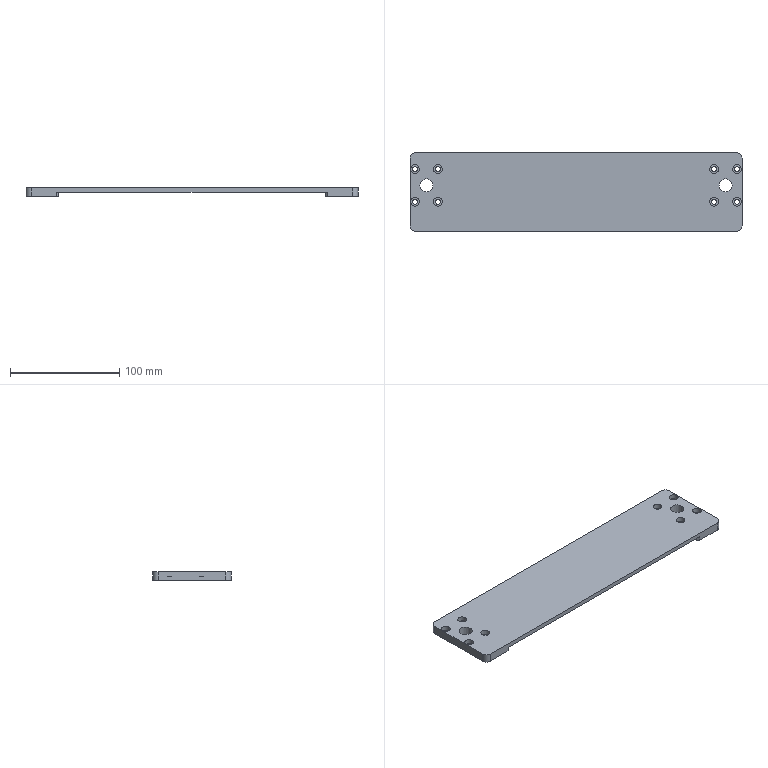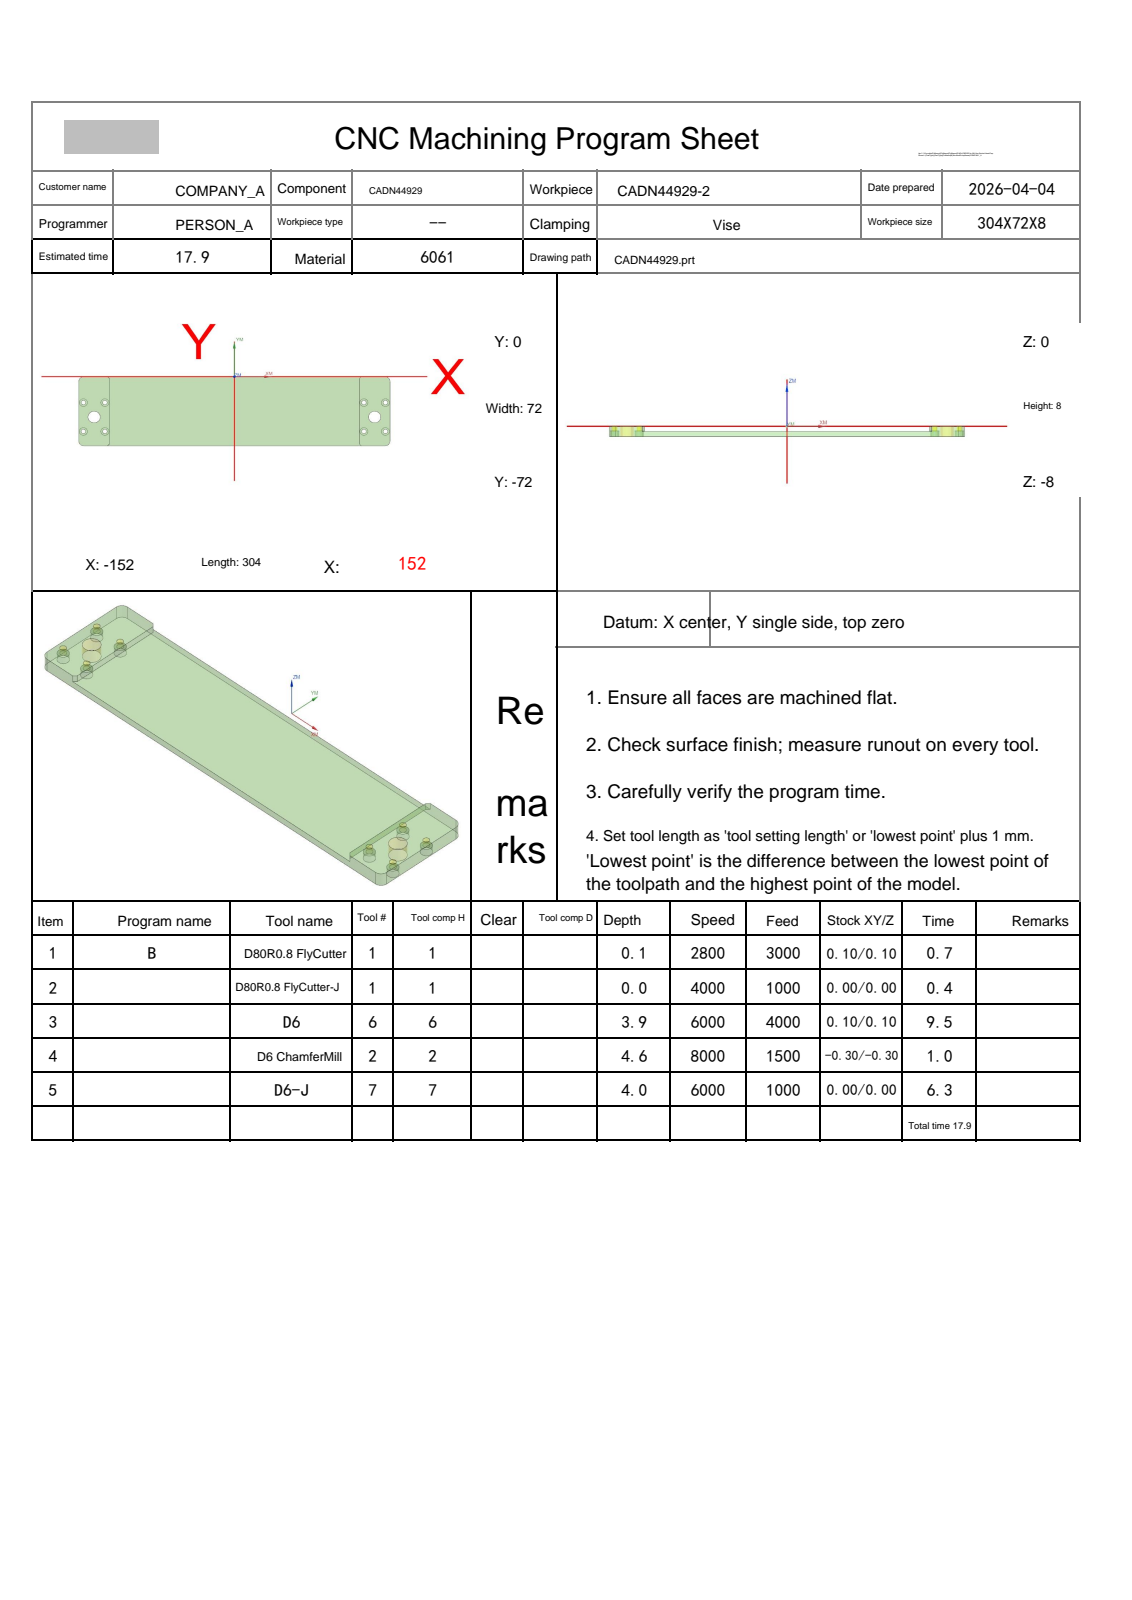NC program | NX | posted by the shop | part box 304 x 72 x 8 mm
Whole program, first 1815 of 1961 lines:
%
O0001
(Machine time: 18.92 MIN)
(===Total Tool:4===)
(T1=D80R0.8 FlyCutter D=80.  R=0.8  D-  H01 Z=0.    )
(T6=D6      D=6.   R=0.   D-  H06 Z=-3.9  )
(T2=D6 ChamferMill   D=6.   R=0.   D-  H02 Z=-4.6  )
(T7=D6-J    D=6.   R=0.   D7  H07 Z=-4.   )
G80 G90 G17 G49 G40
G91 G28 Z0
M01
N1 T01 M06
(D80R0.8 FlyCutter  D=80. R=0.8 H=01 ce=0.10 di=0.10)
G00 G90 G54 X204.097 Y-36. M03 S2800
G43 H01 Z20.
M08
Z3.525
G01 Z1.525 F3000.
X192.097
X-192.097
X-204.097
Z3.525
G00 X204.097
Z3.05
G01 Z1.05
X192.097
X-192.097
X-204.097
Z3.05
G00 X204.097
Z2.575
G01 Z.575
X192.097
X-192.097
X-204.097
Z2.575
G00 X204.097
Z2.1
G01 Z.1
X192.097
X-192.097
X-204.097
Z2.1
G00 Z20.
G91 G28 Z0.0
M05
M09
G91 G28 Z0.0
M01
N2 T01 M06
(D80R0.8 FlyCutter-J  D=80. R=0.8 H=01 ce=0.00 di=0.00)
G00 G90 G54 X203.999 Y-36. M03 S4000
G43 H01 Z20.
M08
Z2.
G01 Z0.0 F1000.
X191.999
X-191.999
X-203.999
Z2.
G00 Z20.
G91 G28 Z0.0
M05
M09
G91 G28 Z0.0
M01
N3 T06 M06
(D6  D=6. R=0. H=06 ce=0.10 di=0.10)
G00 G90 G54 X0.0 Y-78. M03 S6000
G43 H06 Z11.8
M08
Z1.013
G01 Z-.488 F4000.
Y-74.94
X-122.556
X-118.9 Y-71.284
Y-.716
X-122.556 Y2.94
X122.556
X118.9 Y-.716
Y-71.284
X122.556 Y-74.94
X1.821
G02 X1.322 Y-74.673 I.001 J.6
G01 X-1.322 Y-70.707
G03 X-1.82 Y-70.44 I-.499 J-.333
G01 X-113.803
G02 X-114.4 Y-69.843 I.003 J.6
G01 Y-2.157
G02 X-113.803 Y-1.56 I.6 J-.003
G01 X113.803
G02 X114.4 Y-2.157 I-.003 J-.6
G01 Y-69.843
G02 X113.803 Y-70.44 I-.6 J.003
G01 X1.821
G02 X1.322 Y-70.173 I.001 J.6
G01 X-1.322 Y-66.207
G03 X-1.821 Y-65.94 I-.499 J-.333
G01 X-109.303
G02 X-109.9 Y-65.343 I.003 J.6
G01 Y-6.657
G02 X-109.303 Y-6.06 I.6 J-.003
G01 X109.303
G02 X109.9 Y-6.657 I-.003 J-.6
G01 Y-65.343
G02 X109.303 Y-65.94 I-.6 J.003
G01 X1.821
G02 X1.322 Y-65.673 I.001 J.6
G01 X-1.322 Y-61.707
G03 X-1.821 Y-61.44 I-.499 J-.333
G01 X-104.804
G02 X-105.4 Y-60.844 I.004 J.6
G01 Y-11.156
G02 X-104.804 Y-10.56 I.6 J-.004
G01 X104.804
G02 X105.4 Y-11.156 I-.004 J-.6
G01 Y-60.844
G02 X104.804 Y-61.44 I-.6 J.004
G01 X1.821
G02 X1.322 Y-61.173 I.001 J.6
G01 X-1.322 Y-57.207
G03 X-1.821 Y-56.94 I-.499 J-.333
G01 X-100.304
G02 X-100.9 Y-56.344 I.004 J.6
G01 Y-15.656
G02 X-100.304 Y-15.06 I.6 J-.004
G01 X100.304
G02 X100.9 Y-15.656 I-.004 J-.6
G01 Y-56.344
G02 X100.304 Y-56.94 I-.6 J.004
G01 X1.821
G02 X1.322 Y-56.673 I.001 J.6
G01 X-1.322 Y-52.707
G03 X-1.821 Y-52.44 I-.499 J-.333
G01 X-95.804
G02 X-96.4 Y-51.844 I.004 J.6
G01 Y-20.156
G02 X-95.804 Y-19.56 I.6 J-.004
G01 X95.804
G02 X96.4 Y-20.156 I-.004 J-.6
G01 Y-51.844
G02 X95.804 Y-52.44 I-.6 J.004
G01 X1.821
G02 X1.322 Y-52.173 I.001 J.6
G01 X-1.322 Y-48.207
G03 X-1.821 Y-47.94 I-.499 J-.333
G01 X-91.305
G02 X-91.9 Y-47.345 I.005 J.6
G01 Y-24.655
G02 X-91.305 Y-24.06 I.6 J-.004
G01 X91.305
G02 X91.9 Y-24.655 I-.005 J-.6
G01 Y-47.345
G02 X91.305 Y-47.94 I-.6 J.004
G01 X1.821
G02 X1.322 Y-47.673 I.001 J.6
G01 X-1.322 Y-43.707
G03 X-1.821 Y-43.44 I-.499 J-.333
G01 X-86.805
G02 X-87.4 Y-42.845 I.005 J.6
G01 Y-29.155
G02 X-86.805 Y-28.56 I.6 J-.005
G01 X86.805
G02 X87.4 Y-29.155 I-.005 J-.6
G01 Y-42.845
G02 X86.805 Y-43.44 I-.6 J.005
G01 X1.821
G02 X1.322 Y-43.173 I.001 J.6
G01 X-1.322 Y-39.207
G03 X-1.821 Y-38.94 I-.499 J-.333
G01 X-82.305
G02 X-82.9 Y-38.345 I.005 J.6
G01 Y-33.655
G02 X-82.305 Y-33.06 I.6 J-.005
G01 X82.305
G02 X82.9 Y-33.655 I-.005 J-.6
G01 Y-38.345
G02 X82.305 Y-38.94 I-.6 J.005
G01 X1.598
G02 X1.175 Y-38.765 I.001 J.6
G01 X-1.174 Y-36.416
G03 X-1.599 Y-36.24 I-.424 J-.424
G01 X-79.963
G02 X-80.2 Y-36. I.003 J.24
G01 Y-35.997
G02 X-79.963 Y-35.76 I.24 J-.003
G01 X79.963
G02 X80.2 Y-36. I-.003 J-.24
G01 Y-36.003
G02 X79.963 Y-36.24 I-.24 J.003
G01 X0.0
X-.5
Y-39.24
Z1.013
G00 X0.0 Y-78.
Z.525
G01 Z-.975
Y-74.94
X-122.556
X-118.9 Y-71.284
Y-.716
X-122.556 Y2.94
X122.556
X118.9 Y-.716
Y-71.284
X122.556 Y-74.94
X1.821
G02 X1.322 Y-74.673 I.001 J.6
G01 X-1.322 Y-70.707
G03 X-1.82 Y-70.44 I-.499 J-.333
G01 X-113.803
G02 X-114.4 Y-69.843 I.003 J.6
G01 Y-2.157
G02 X-113.803 Y-1.56 I.6 J-.003
G01 X113.803
G02 X114.4 Y-2.157 I-.003 J-.6
G01 Y-69.843
G02 X113.803 Y-70.44 I-.6 J.003
G01 X1.821
G02 X1.322 Y-70.173 I.001 J.6
G01 X-1.322 Y-66.207
G03 X-1.821 Y-65.94 I-.499 J-.333
G01 X-109.303
G02 X-109.9 Y-65.343 I.003 J.6
G01 Y-6.657
G02 X-109.303 Y-6.06 I.6 J-.003
G01 X109.303
G02 X109.9 Y-6.657 I-.003 J-.6
G01 Y-65.343
G02 X109.303 Y-65.94 I-.6 J.003
G01 X1.821
G02 X1.322 Y-65.673 I.001 J.6
G01 X-1.322 Y-61.707
G03 X-1.821 Y-61.44 I-.499 J-.333
G01 X-104.804
G02 X-105.4 Y-60.844 I.004 J.6
G01 Y-11.156
G02 X-104.804 Y-10.56 I.6 J-.004
G01 X104.804
G02 X105.4 Y-11.156 I-.004 J-.6
G01 Y-60.844
G02 X104.804 Y-61.44 I-.6 J.004
G01 X1.821
G02 X1.322 Y-61.173 I.001 J.6
G01 X-1.322 Y-57.207
G03 X-1.821 Y-56.94 I-.499 J-.333
G01 X-100.304
G02 X-100.9 Y-56.344 I.004 J.6
G01 Y-15.656
G02 X-100.304 Y-15.06 I.6 J-.004
G01 X100.304
G02 X100.9 Y-15.656 I-.004 J-.6
G01 Y-56.344
G02 X100.304 Y-56.94 I-.6 J.004
G01 X1.821
G02 X1.322 Y-56.673 I.001 J.6
G01 X-1.322 Y-52.707
G03 X-1.821 Y-52.44 I-.499 J-.333
G01 X-95.804
G02 X-96.4 Y-51.844 I.004 J.6
G01 Y-20.156
G02 X-95.804 Y-19.56 I.6 J-.004
G01 X95.804
G02 X96.4 Y-20.156 I-.004 J-.6
G01 Y-51.844
G02 X95.804 Y-52.44 I-.6 J.004
G01 X1.821
G02 X1.322 Y-52.173 I.001 J.6
G01 X-1.322 Y-48.207
G03 X-1.821 Y-47.94 I-.499 J-.333
G01 X-91.305
G02 X-91.9 Y-47.345 I.005 J.6
G01 Y-24.655
G02 X-91.305 Y-24.06 I.6 J-.004
G01 X91.305
G02 X91.9 Y-24.655 I-.005 J-.6
G01 Y-47.345
G02 X91.305 Y-47.94 I-.6 J.004
G01 X1.821
G02 X1.322 Y-47.673 I.001 J.6
G01 X-1.322 Y-43.707
G03 X-1.821 Y-43.44 I-.499 J-.333
G01 X-86.805
G02 X-87.4 Y-42.845 I.005 J.6
G01 Y-29.155
G02 X-86.805 Y-28.56 I.6 J-.005
G01 X86.805
G02 X87.4 Y-29.155 I-.005 J-.6
G01 Y-42.845
G02 X86.805 Y-43.44 I-.6 J.005
G01 X1.821
G02 X1.322 Y-43.173 I.001 J.6
G01 X-1.322 Y-39.207
G03 X-1.821 Y-38.94 I-.499 J-.333
G01 X-82.305
G02 X-82.9 Y-38.345 I.005 J.6
G01 Y-33.655
G02 X-82.305 Y-33.06 I.6 J-.005
G01 X82.305
G02 X82.9 Y-33.655 I-.005 J-.6
G01 Y-38.345
G02 X82.305 Y-38.94 I-.6 J.005
G01 X1.598
G02 X1.175 Y-38.765 I.001 J.6
G01 X-1.174 Y-36.416
G03 X-1.599 Y-36.24 I-.424 J-.424
G01 X-79.963
G02 X-80.2 Y-36. I.003 J.24
G01 Y-35.997
G02 X-79.963 Y-35.76 I.24 J-.003
G01 X79.963
G02 X80.2 Y-36. I-.003 J-.24
G01 Y-36.003
G02 X79.963 Y-36.24 I-.24 J.003
G01 X0.0
X-.5
Y-39.24
Z.525
G00 X0.0 Y-78.
Z.038
G01 Z-1.463
Y-74.94
X-122.556
X-118.9 Y-71.284
Y-.716
X-122.556 Y2.94
X122.556
X118.9 Y-.716
Y-71.284
X122.556 Y-74.94
X1.821
G02 X1.322 Y-74.673 I.001 J.6
G01 X-1.322 Y-70.707
G03 X-1.82 Y-70.44 I-.499 J-.333
G01 X-113.803
G02 X-114.4 Y-69.843 I.003 J.6
G01 Y-2.157
G02 X-113.803 Y-1.56 I.6 J-.003
G01 X113.803
G02 X114.4 Y-2.157 I-.003 J-.6
G01 Y-69.843
G02 X113.803 Y-70.44 I-.6 J.003
G01 X1.821
G02 X1.322 Y-70.173 I.001 J.6
G01 X-1.322 Y-66.207
G03 X-1.821 Y-65.94 I-.499 J-.333
G01 X-109.303
G02 X-109.9 Y-65.343 I.003 J.6
G01 Y-6.657
G02 X-109.303 Y-6.06 I.6 J-.003
G01 X109.303
G02 X109.9 Y-6.657 I-.003 J-.6
G01 Y-65.343
G02 X109.303 Y-65.94 I-.6 J.003
G01 X1.821
G02 X1.322 Y-65.673 I.001 J.6
G01 X-1.322 Y-61.707
G03 X-1.821 Y-61.44 I-.499 J-.333
G01 X-104.804
G02 X-105.4 Y-60.844 I.004 J.6
G01 Y-11.156
G02 X-104.804 Y-10.56 I.6 J-.004
G01 X104.804
G02 X105.4 Y-11.156 I-.004 J-.6
G01 Y-60.844
G02 X104.804 Y-61.44 I-.6 J.004
G01 X1.821
G02 X1.322 Y-61.173 I.001 J.6
G01 X-1.322 Y-57.207
G03 X-1.821 Y-56.94 I-.499 J-.333
G01 X-100.304
G02 X-100.9 Y-56.344 I.004 J.6
G01 Y-15.656
G02 X-100.304 Y-15.06 I.6 J-.004
G01 X100.304
G02 X100.9 Y-15.656 I-.004 J-.6
G01 Y-56.344
G02 X100.304 Y-56.94 I-.6 J.004
G01 X1.821
G02 X1.322 Y-56.673 I.001 J.6
G01 X-1.322 Y-52.707
G03 X-1.821 Y-52.44 I-.499 J-.333
G01 X-95.804
G02 X-96.4 Y-51.844 I.004 J.6
G01 Y-20.156
G02 X-95.804 Y-19.56 I.6 J-.004
G01 X95.804
G02 X96.4 Y-20.156 I-.004 J-.6
G01 Y-51.844
G02 X95.804 Y-52.44 I-.6 J.004
G01 X1.821
G02 X1.322 Y-52.173 I.001 J.6
G01 X-1.322 Y-48.207
G03 X-1.821 Y-47.94 I-.499 J-.333
G01 X-91.305
G02 X-91.9 Y-47.345 I.005 J.6
G01 Y-24.655
G02 X-91.305 Y-24.06 I.6 J-.004
G01 X91.305
G02 X91.9 Y-24.655 I-.005 J-.6
G01 Y-47.345
G02 X91.305 Y-47.94 I-.6 J.004
G01 X1.821
G02 X1.322 Y-47.673 I.001 J.6
G01 X-1.322 Y-43.707
G03 X-1.821 Y-43.44 I-.499 J-.333
G01 X-86.805
G02 X-87.4 Y-42.845 I.005 J.6
G01 Y-29.155
G02 X-86.805 Y-28.56 I.6 J-.005
G01 X86.805
G02 X87.4 Y-29.155 I-.005 J-.6
G01 Y-42.845
G02 X86.805 Y-43.44 I-.6 J.005
G01 X1.821
G02 X1.322 Y-43.173 I.001 J.6
G01 X-1.322 Y-39.207
G03 X-1.821 Y-38.94 I-.499 J-.333
G01 X-82.305
G02 X-82.9 Y-38.345 I.005 J.6
G01 Y-33.655
G02 X-82.305 Y-33.06 I.6 J-.005
G01 X82.305
G02 X82.9 Y-33.655 I-.005 J-.6
G01 Y-38.345
G02 X82.305 Y-38.94 I-.6 J.005
G01 X1.598
G02 X1.175 Y-38.765 I.001 J.6
G01 X-1.174 Y-36.416
G03 X-1.599 Y-36.24 I-.424 J-.424
G01 X-79.963
G02 X-80.2 Y-36. I.003 J.24
G01 Y-35.997
G02 X-79.963 Y-35.76 I.24 J-.003
G01 X79.963
G02 X80.2 Y-36. I-.003 J-.24
G01 Y-36.003
G02 X79.963 Y-36.24 I-.24 J.003
G01 X0.0
X-.5
Y-39.24
Z.038
G00 X0.0 Y-78.
Z-.45
G01 Z-1.95
Y-74.94
X-122.556
X-118.9 Y-71.284
Y-.716
X-122.556 Y2.94
X122.556
X118.9 Y-.716
Y-71.284
X122.556 Y-74.94
X1.821
G02 X1.322 Y-74.673 I.001 J.6
G01 X-1.322 Y-70.707
G03 X-1.82 Y-70.44 I-.499 J-.333
G01 X-113.803
G02 X-114.4 Y-69.843 I.003 J.6
G01 Y-2.157
G02 X-113.803 Y-1.56 I.6 J-.003
G01 X113.803
G02 X114.4 Y-2.157 I-.003 J-.6
G01 Y-69.843
G02 X113.803 Y-70.44 I-.6 J.003
G01 X1.821
G02 X1.322 Y-70.173 I.001 J.6
G01 X-1.322 Y-66.207
G03 X-1.821 Y-65.94 I-.499 J-.333
G01 X-109.303
G02 X-109.9 Y-65.343 I.003 J.6
G01 Y-6.657
G02 X-109.303 Y-6.06 I.6 J-.003
G01 X109.303
G02 X109.9 Y-6.657 I-.003 J-.6
G01 Y-65.343
G02 X109.303 Y-65.94 I-.6 J.003
G01 X1.821
G02 X1.322 Y-65.673 I.001 J.6
G01 X-1.322 Y-61.707
G03 X-1.821 Y-61.44 I-.499 J-.333
G01 X-104.804
G02 X-105.4 Y-60.844 I.004 J.6
G01 Y-11.156
G02 X-104.804 Y-10.56 I.6 J-.004
G01 X104.804
G02 X105.4 Y-11.156 I-.004 J-.6
G01 Y-60.844
G02 X104.804 Y-61.44 I-.6 J.004
G01 X1.821
G02 X1.322 Y-61.173 I.001 J.6
G01 X-1.322 Y-57.207
G03 X-1.821 Y-56.94 I-.499 J-.333
G01 X-100.304
G02 X-100.9 Y-56.344 I.004 J.6
G01 Y-15.656
G02 X-100.304 Y-15.06 I.6 J-.004
G01 X100.304
G02 X100.9 Y-15.656 I-.004 J-.6
G01 Y-56.344
G02 X100.304 Y-56.94 I-.6 J.004
G01 X1.821
G02 X1.322 Y-56.673 I.001 J.6
G01 X-1.322 Y-52.707
G03 X-1.821 Y-52.44 I-.499 J-.333
G01 X-95.804
G02 X-96.4 Y-51.844 I.004 J.6
G01 Y-20.156
G02 X-95.804 Y-19.56 I.6 J-.004
G01 X95.804
G02 X96.4 Y-20.156 I-.004 J-.6
G01 Y-51.844
G02 X95.804 Y-52.44 I-.6 J.004
G01 X1.821
G02 X1.322 Y-52.173 I.001 J.6
G01 X-1.322 Y-48.207
G03 X-1.821 Y-47.94 I-.499 J-.333
G01 X-91.305
G02 X-91.9 Y-47.345 I.005 J.6
G01 Y-24.655
G02 X-91.305 Y-24.06 I.6 J-.004
G01 X91.305
G02 X91.9 Y-24.655 I-.005 J-.6
G01 Y-47.345
G02 X91.305 Y-47.94 I-.6 J.004
G01 X1.821
G02 X1.322 Y-47.673 I.001 J.6
G01 X-1.322 Y-43.707
G03 X-1.821 Y-43.44 I-.499 J-.333
G01 X-86.805
G02 X-87.4 Y-42.845 I.005 J.6
G01 Y-29.155
G02 X-86.805 Y-28.56 I.6 J-.005
G01 X86.805
G02 X87.4 Y-29.155 I-.005 J-.6
G01 Y-42.845
G02 X86.805 Y-43.44 I-.6 J.005
G01 X1.821
G02 X1.322 Y-43.173 I.001 J.6
G01 X-1.322 Y-39.207
G03 X-1.821 Y-38.94 I-.499 J-.333
G01 X-82.305
G02 X-82.9 Y-38.345 I.005 J.6
G01 Y-33.655
G02 X-82.305 Y-33.06 I.6 J-.005
G01 X82.305
G02 X82.9 Y-33.655 I-.005 J-.6
G01 Y-38.345
G02 X82.305 Y-38.94 I-.6 J.005
G01 X1.598
G02 X1.175 Y-38.765 I.001 J.6
G01 X-1.174 Y-36.416
G03 X-1.599 Y-36.24 I-.424 J-.424
G01 X-79.963
G02 X-80.2 Y-36. I.003 J.24
G01 Y-35.997
G02 X-79.963 Y-35.76 I.24 J-.003
G01 X79.963
G02 X80.2 Y-36. I-.003 J-.24
G01 Y-36.003
G02 X79.963 Y-36.24 I-.24 J.003
G01 X0.0
X-.5
Y-39.24
Z-.45
G00 X0.0 Y-78.
Z-.938
G01 Z-2.438
Y-74.94
X-122.556
X-118.9 Y-71.284
Y-.716
X-122.556 Y2.94
X122.556
X118.9 Y-.716
Y-71.284
X122.556 Y-74.94
X1.821
G02 X1.322 Y-74.673 I.001 J.6
G01 X-1.322 Y-70.707
G03 X-1.82 Y-70.44 I-.499 J-.333
G01 X-113.803
G02 X-114.4 Y-69.843 I.003 J.6
G01 Y-2.157
G02 X-113.803 Y-1.56 I.6 J-.003
G01 X113.803
G02 X114.4 Y-2.157 I-.003 J-.6
G01 Y-69.843
G02 X113.803 Y-70.44 I-.6 J.003
G01 X1.821
G02 X1.322 Y-70.173 I.001 J.6
G01 X-1.322 Y-66.207
G03 X-1.821 Y-65.94 I-.499 J-.333
G01 X-109.303
G02 X-109.9 Y-65.343 I.003 J.6
G01 Y-6.657
G02 X-109.303 Y-6.06 I.6 J-.003
G01 X109.303
G02 X109.9 Y-6.657 I-.003 J-.6
G01 Y-65.343
G02 X109.303 Y-65.94 I-.6 J.003
G01 X1.821
G02 X1.322 Y-65.673 I.001 J.6
G01 X-1.322 Y-61.707
G03 X-1.821 Y-61.44 I-.499 J-.333
G01 X-104.804
G02 X-105.4 Y-60.844 I.004 J.6
G01 Y-11.156
G02 X-104.804 Y-10.56 I.6 J-.004
G01 X104.804
G02 X105.4 Y-11.156 I-.004 J-.6
G01 Y-60.844
G02 X104.804 Y-61.44 I-.6 J.004
G01 X1.821
G02 X1.322 Y-61.173 I.001 J.6
G01 X-1.322 Y-57.207
G03 X-1.821 Y-56.94 I-.499 J-.333
G01 X-100.304
G02 X-100.9 Y-56.344 I.004 J.6
G01 Y-15.656
G02 X-100.304 Y-15.06 I.6 J-.004
G01 X100.304
G02 X100.9 Y-15.656 I-.004 J-.6
G01 Y-56.344
G02 X100.304 Y-56.94 I-.6 J.004
G01 X1.821
G02 X1.322 Y-56.673 I.001 J.6
G01 X-1.322 Y-52.707
G03 X-1.821 Y-52.44 I-.499 J-.333
G01 X-95.804
G02 X-96.4 Y-51.844 I.004 J.6
G01 Y-20.156
G02 X-95.804 Y-19.56 I.6 J-.004
G01 X95.804
G02 X96.4 Y-20.156 I-.004 J-.6
G01 Y-51.844
G02 X95.804 Y-52.44 I-.6 J.004
G01 X1.821
G02 X1.322 Y-52.173 I.001 J.6
G01 X-1.322 Y-48.207
G03 X-1.821 Y-47.94 I-.499 J-.333
G01 X-91.305
G02 X-91.9 Y-47.345 I.005 J.6
G01 Y-24.655
G02 X-91.305 Y-24.06 I.6 J-.004
G01 X91.305
G02 X91.9 Y-24.655 I-.005 J-.6
G01 Y-47.345
G02 X91.305 Y-47.94 I-.6 J.004
G01 X1.821
G02 X1.322 Y-47.673 I.001 J.6
G01 X-1.322 Y-43.707
G03 X-1.821 Y-43.44 I-.499 J-.333
G01 X-86.805
G02 X-87.4 Y-42.845 I.005 J.6
G01 Y-29.155
G02 X-86.805 Y-28.56 I.6 J-.005
G01 X86.805
G02 X87.4 Y-29.155 I-.005 J-.6
G01 Y-42.845
G02 X86.805 Y-43.44 I-.6 J.005
G01 X1.821
G02 X1.322 Y-43.173 I.001 J.6
G01 X-1.322 Y-39.207
G03 X-1.821 Y-38.94 I-.499 J-.333
G01 X-82.305
G02 X-82.9 Y-38.345 I.005 J.6
G01 Y-33.655
G02 X-82.305 Y-33.06 I.6 J-.005
G01 X82.305
G02 X82.9 Y-33.655 I-.005 J-.6
G01 Y-38.345
G02 X82.305 Y-38.94 I-.6 J.005
G01 X1.598
G02 X1.175 Y-38.765 I.001 J.6
G01 X-1.174 Y-36.416
G03 X-1.599 Y-36.24 I-.424 J-.424
G01 X-79.963
G02 X-80.2 Y-36. I.003 J.24
G01 Y-35.997
G02 X-79.963 Y-35.76 I.24 J-.003
G01 X79.963
G02 X80.2 Y-36. I-.003 J-.24
G01 Y-36.003
G02 X79.963 Y-36.24 I-.24 J.003
G01 X0.0
X-.5
Y-39.24
Z-.938
G00 X0.0 Y-78.
Z-1.425
G01 Z-2.925
Y-74.94
X-122.556
X-118.9 Y-71.284
Y-.716
X-122.556 Y2.94
X122.556
X118.9 Y-.716
Y-71.284
X122.556 Y-74.94
X1.821
G02 X1.322 Y-74.673 I.001 J.6
G01 X-1.322 Y-70.707
G03 X-1.82 Y-70.44 I-.499 J-.333
G01 X-113.803
G02 X-114.4 Y-69.843 I.003 J.6
G01 Y-2.157
G02 X-113.803 Y-1.56 I.6 J-.003
G01 X113.803
G02 X114.4 Y-2.157 I-.003 J-.6
G01 Y-69.843
G02 X113.803 Y-70.44 I-.6 J.003
G01 X1.821
G02 X1.322 Y-70.173 I.001 J.6
G01 X-1.322 Y-66.207
G03 X-1.821 Y-65.94 I-.499 J-.333
G01 X-109.303
G02 X-109.9 Y-65.343 I.003 J.6
G01 Y-6.657
G02 X-109.303 Y-6.06 I.6 J-.003
G01 X109.303
G02 X109.9 Y-6.657 I-.003 J-.6
G01 Y-65.343
G02 X109.303 Y-65.94 I-.6 J.003
G01 X1.821
G02 X1.322 Y-65.673 I.001 J.6
G01 X-1.322 Y-61.707
G03 X-1.821 Y-61.44 I-.499 J-.333
G01 X-104.804
G02 X-105.4 Y-60.844 I.004 J.6
G01 Y-11.156
G02 X-104.804 Y-10.56 I.6 J-.004
G01 X104.804
G02 X105.4 Y-11.156 I-.004 J-.6
G01 Y-60.844
G02 X104.804 Y-61.44 I-.6 J.004
G01 X1.821
G02 X1.322 Y-61.173 I.001 J.6
G01 X-1.322 Y-57.207
G03 X-1.821 Y-56.94 I-.499 J-.333
G01 X-100.304
G02 X-100.9 Y-56.344 I.004 J.6
G01 Y-15.656
G02 X-100.304 Y-15.06 I.6 J-.004
G01 X100.304
G02 X100.9 Y-15.656 I-.004 J-.6
G01 Y-56.344
G02 X100.304 Y-56.94 I-.6 J.004
G01 X1.821
G02 X1.322 Y-56.673 I.001 J.6
G01 X-1.322 Y-52.707
G03 X-1.821 Y-52.44 I-.499 J-.333
G01 X-95.804
G02 X-96.4 Y-51.844 I.004 J.6
G01 Y-20.156
G02 X-95.804 Y-19.56 I.6 J-.004
G01 X95.804
G02 X96.4 Y-20.156 I-.004 J-.6
G01 Y-51.844
G02 X95.804 Y-52.44 I-.6 J.004
G01 X1.821
G02 X1.322 Y-52.173 I.001 J.6
G01 X-1.322 Y-48.207
G03 X-1.821 Y-47.94 I-.499 J-.333
G01 X-91.305
G02 X-91.9 Y-47.345 I.005 J.6
G01 Y-24.655
G02 X-91.305 Y-24.06 I.6 J-.004
G01 X91.305
G02 X91.9 Y-24.655 I-.005 J-.6
G01 Y-47.345
G02 X91.305 Y-47.94 I-.6 J.004
G01 X1.821
G02 X1.322 Y-47.673 I.001 J.6
G01 X-1.322 Y-43.707
G03 X-1.821 Y-43.44 I-.499 J-.333
G01 X-86.805
G02 X-87.4 Y-42.845 I.005 J.6
G01 Y-29.155
G02 X-86.805 Y-28.56 I.6 J-.005
G01 X86.805
G02 X87.4 Y-29.155 I-.005 J-.6
G01 Y-42.845
G02 X86.805 Y-43.44 I-.6 J.005
G01 X1.821
G02 X1.322 Y-43.173 I.001 J.6
G01 X-1.322 Y-39.207
G03 X-1.821 Y-38.94 I-.499 J-.333
G01 X-82.305
G02 X-82.9 Y-38.345 I.005 J.6
G01 Y-33.655
G02 X-82.305 Y-33.06 I.6 J-.005
G01 X82.305
G02 X82.9 Y-33.655 I-.005 J-.6
G01 Y-38.345
G02 X82.305 Y-38.94 I-.6 J.005
G01 X1.598
G02 X1.175 Y-38.765 I.001 J.6
G01 X-1.174 Y-36.416
G03 X-1.599 Y-36.24 I-.424 J-.424
G01 X-79.963
G02 X-80.2 Y-36. I.003 J.24
G01 Y-35.997
G02 X-79.963 Y-35.76 I.24 J-.003
G01 X79.963
G02 X80.2 Y-36. I-.003 J-.24
G01 Y-36.003
G02 X79.963 Y-36.24 I-.24 J.003
G01 X0.0
X-.5
Y-39.24
Z-1.425
G00 X0.0 Y-78.
Z-1.913
G01 Z-3.413
Y-74.94
X-122.556
X-118.9 Y-71.284
Y-.716
X-122.556 Y2.94
X122.556
X118.9 Y-.716
Y-71.284
X122.556 Y-74.94
X1.821
G02 X1.322 Y-74.673 I.001 J.6
G01 X-1.322 Y-70.707
G03 X-1.82 Y-70.44 I-.499 J-.333
G01 X-113.803
G02 X-114.4 Y-69.843 I.003 J.6
G01 Y-2.157
G02 X-113.803 Y-1.56 I.6 J-.003
G01 X113.803
G02 X114.4 Y-2.157 I-.003 J-.6
G01 Y-69.843
G02 X113.803 Y-70.44 I-.6 J.003
G01 X1.821
G02 X1.322 Y-70.173 I.001 J.6
G01 X-1.322 Y-66.207
G03 X-1.821 Y-65.94 I-.499 J-.333
G01 X-109.303
G02 X-109.9 Y-65.343 I.003 J.6
G01 Y-6.657
G02 X-109.303 Y-6.06 I.6 J-.003
G01 X109.303
G02 X109.9 Y-6.657 I-.003 J-.6
G01 Y-65.343
G02 X109.303 Y-65.94 I-.6 J.003
G01 X1.821
G02 X1.322 Y-65.673 I.001 J.6
G01 X-1.322 Y-61.707
G03 X-1.821 Y-61.44 I-.499 J-.333
G01 X-104.804
G02 X-105.4 Y-60.844 I.004 J.6
G01 Y-11.156
G02 X-104.804 Y-10.56 I.6 J-.004
G01 X104.804
G02 X105.4 Y-11.156 I-.004 J-.6
G01 Y-60.844
G02 X104.804 Y-61.44 I-.6 J.004
G01 X1.821
G02 X1.322 Y-61.173 I.001 J.6
G01 X-1.322 Y-57.207
G03 X-1.821 Y-56.94 I-.499 J-.333
G01 X-100.304
G02 X-100.9 Y-56.344 I.004 J.6
G01 Y-15.656
G02 X-100.304 Y-15.06 I.6 J-.004
G01 X100.304
G02 X100.9 Y-15.656 I-.004 J-.6
G01 Y-56.344
G02 X100.304 Y-56.94 I-.6 J.004
G01 X1.821
G02 X1.322 Y-56.673 I.001 J.6
G01 X-1.322 Y-52.707
G03 X-1.821 Y-52.44 I-.499 J-.333
G01 X-95.804
G02 X-96.4 Y-51.844 I.004 J.6
G01 Y-20.156
G02 X-95.804 Y-19.56 I.6 J-.004
G01 X95.804
G02 X96.4 Y-20.156 I-.004 J-.6
G01 Y-51.844
G02 X95.804 Y-52.44 I-.6 J.004
G01 X1.821
G02 X1.322 Y-52.173 I.001 J.6
G01 X-1.322 Y-48.207
G03 X-1.821 Y-47.94 I-.499 J-.333
G01 X-91.305
G02 X-91.9 Y-47.345 I.005 J.6
G01 Y-24.655
G02 X-91.305 Y-24.06 I.6 J-.004
G01 X91.305
G02 X91.9 Y-24.655 I-.005 J-.6
G01 Y-47.345
G02 X91.305 Y-47.94 I-.6 J.004
G01 X1.821
G02 X1.322 Y-47.673 I.001 J.6
G01 X-1.322 Y-43.707
G03 X-1.821 Y-43.44 I-.499 J-.333
G01 X-86.805
G02 X-87.4 Y-42.845 I.005 J.6
G01 Y-29.155
G02 X-86.805 Y-28.56 I.6 J-.005
G01 X86.805
G02 X87.4 Y-29.155 I-.005 J-.6
G01 Y-42.845
G02 X86.805 Y-43.44 I-.6 J.005
G01 X1.821
G02 X1.322 Y-43.173 I.001 J.6
G01 X-1.322 Y-39.207
G03 X-1.821 Y-38.94 I-.499 J-.333
G01 X-82.305
G02 X-82.9 Y-38.345 I.005 J.6
G01 Y-33.655
G02 X-82.305 Y-33.06 I.6 J-.005
G01 X82.305
G02 X82.9 Y-33.655 I-.005 J-.6
G01 Y-38.345
G02 X82.305 Y-38.94 I-.6 J.005
G01 X1.598
G02 X1.175 Y-38.765 I.001 J.6
G01 X-1.174 Y-36.416
G03 X-1.599 Y-36.24 I-.424 J-.424
G01 X-79.963
G02 X-80.2 Y-36. I.003 J.24
G01 Y-35.997
G02 X-79.963 Y-35.76 I.24 J-.003
G01 X79.963
G02 X80.2 Y-36. I-.003 J-.24
G01 Y-36.003
G02 X79.963 Y-36.24 I-.24 J.003
G01 X0.0
X-.5
Y-39.24
Z-1.913
G00 X0.0 Y-78.
Z-2.4
G01 Z-3.9
Y-74.94
X-122.556
X-118.9 Y-71.284
Y-.716
X-122.556 Y2.94
X122.556
X118.9 Y-.716
Y-71.284
X122.556 Y-74.94
X1.821
G02 X1.322 Y-74.673 I.001 J.6
G01 X-1.322 Y-70.707
G03 X-1.82 Y-70.44 I-.499 J-.333
G01 X-113.803
G02 X-114.4 Y-69.843 I.003 J.6
G01 Y-2.157
G02 X-113.803 Y-1.56 I.6 J-.003
G01 X113.803
G02 X114.4 Y-2.157 I-.003 J-.6
G01 Y-69.843
G02 X113.803 Y-70.44 I-.6 J.003
G01 X1.821
G02 X1.322 Y-70.173 I.001 J.6
G01 X-1.322 Y-66.207
G03 X-1.821 Y-65.94 I-.499 J-.333
G01 X-109.303
G02 X-109.9 Y-65.343 I.003 J.6
G01 Y-6.657
G02 X-109.303 Y-6.06 I.6 J-.003
G01 X109.303
G02 X109.9 Y-6.657 I-.003 J-.6
G01 Y-65.343
G02 X109.303 Y-65.94 I-.6 J.003
G01 X1.821
G02 X1.322 Y-65.673 I.001 J.6
G01 X-1.322 Y-61.707
G03 X-1.821 Y-61.44 I-.499 J-.333
G01 X-104.804
G02 X-105.4 Y-60.844 I.004 J.6
G01 Y-11.156
G02 X-104.804 Y-10.56 I.6 J-.004
G01 X104.804
G02 X105.4 Y-11.156 I-.004 J-.6
G01 Y-60.844
G02 X104.804 Y-61.44 I-.6 J.004
G01 X1.821
G02 X1.322 Y-61.173 I.001 J.6
G01 X-1.322 Y-57.207
G03 X-1.821 Y-56.94 I-.499 J-.333
G01 X-100.304
G02 X-100.9 Y-56.344 I.004 J.6
G01 Y-15.656
G02 X-100.304 Y-15.06 I.6 J-.004
G01 X100.304
G02 X100.9 Y-15.656 I-.004 J-.6
G01 Y-56.344
G02 X100.304 Y-56.94 I-.6 J.004
G01 X1.821
G02 X1.322 Y-56.673 I.001 J.6
G01 X-1.322 Y-52.707
G03 X-1.821 Y-52.44 I-.499 J-.333
G01 X-95.804
G02 X-96.4 Y-51.844 I.004 J.6
G01 Y-20.156
G02 X-95.804 Y-19.56 I.6 J-.004
G01 X95.804
G02 X96.4 Y-20.156 I-.004 J-.6
G01 Y-51.844
G02 X95.804 Y-52.44 I-.6 J.004
G01 X1.821
G02 X1.322 Y-52.173 I.001 J.6
G01 X-1.322 Y-48.207
G03 X-1.821 Y-47.94 I-.499 J-.333
G01 X-91.305
G02 X-91.9 Y-47.345 I.005 J.6
G01 Y-24.655
G02 X-91.305 Y-24.06 I.6 J-.004
G01 X91.305
G02 X91.9 Y-24.655 I-.005 J-.6
G01 Y-47.345
G02 X91.305 Y-47.94 I-.6 J.004
G01 X1.821
G02 X1.322 Y-47.673 I.001 J.6
G01 X-1.322 Y-43.707
G03 X-1.821 Y-43.44 I-.499 J-.333
G01 X-86.805
G02 X-87.4 Y-42.845 I.005 J.6
G01 Y-29.155
G02 X-86.805 Y-28.56 I.6 J-.005
G01 X86.805
G02 X87.4 Y-29.155 I-.005 J-.6
G01 Y-42.845
G02 X86.805 Y-43.44 I-.6 J.005
G01 X1.821
G02 X1.322 Y-43.173 I.001 J.6
G01 X-1.322 Y-39.207
G03 X-1.821 Y-38.94 I-.499 J-.333
G01 X-82.305
G02 X-82.9 Y-38.345 I.005 J.6
G01 Y-33.655
G02 X-82.305 Y-33.06 I.6 J-.005
G01 X82.305
G02 X82.9 Y-33.655 I-.005 J-.6
G01 Y-38.345
G02 X82.305 Y-38.94 I-.6 J.005
G01 X1.598
G02 X1.175 Y-38.765 I.001 J.6
G01 X-1.174 Y-36.416
G03 X-1.599 Y-36.24 I-.424 J-.424
G01 X-79.963
G02 X-80.2 Y-36. I.003 J.24
G01 Y-35.997
G02 X-79.963 Y-35.76 I.24 J-.003
G01 X79.963
G02 X80.2 Y-36. I-.003 J-.24
G01 Y-36.003
G02 X79.963 Y-36.24 I-.24 J.003
G01 X0.0
X-.5
Y-39.24
Z-2.4
G00 Z11.8
G91 G28 Z0.0
M05
M09
G91 G28 Z0.0
M01
N4 T02 M06
(D6 ChamferMill  D=6. R=0. H=02 ce=0.00 di=0.10)
G00 G90 G54 X-126.5 Y-27. M03 S8000
G43 H02 Z20.
M08
G98 G81 X-126.5 Y-27. Z-2.55 R3. F1000.
X-147.5
Y-57.
X-126.5
X126.5
X147.5
Y-27.
X126.5
G80
G00 Z20.
G00 G90 X134.7 Y-39. M03 S8000
Z20.
Z-.5
G01 Z-1. F1200.
G03 X131.7 Y-42. I0.0 J-3.
X137. Y-47.3 I5.3 J0.0
X142.3 Y-42. I0.0 J5.3
X137. Y-36.7 I-5.3 J0.0
X131.7 Y-42. I0.0 J-5.3
X134.7 Y-45. I3. J0.0
G01 Z-.5
G00 Z20.
X-139.3 Y-39.
Z-.5
G01 Z-1.
G03 X-142.3 Y-42. I0.0 J-3.
X-137. Y-47.3 I5.3 J0.0
X-131.7 Y-42. I0.0 J5.3
X-137. Y-36.7 I-5.3 J0.0
X-142.3 Y-42. I0.0 J-5.3
X-139.3 Y-45. I3. J0.0
G01 Z-.5
G00 Z20.
G00 G90 X121.373 Y-36.386 M03 S6500
Z20.
Z.772
G01 Z-.6 F1500.
G03 X121.573 Y-36.1 I-1.532 J1.286
G01 X121.603 Y-36.054
X121.6 Y-36.
Y-2.
X121.63 Y-1.847
X121.717 Y-1.717
X123.717 Y.283
X123.847 Y.37
X124. Y.4
X147.
G02 X152.4 Y-5. I0.0 J-5.4
G01 Y-67.
G02 X147. Y-72.4 I-5.4 J0.0
G01 X124.
X123.847 Y-72.37
X123.717 Y-72.283
X121.717 Y-70.283
X121.63 Y-70.153
X121.6 Y-70.
Y-36.
X121.603 Y-35.946
X121.573 Y-35.9
G03 X121.373 Y-35.614 I-1.732 J-1.
G01 Z.772
G00 Z3.15
X124.842 Y-26.596
Z.863
G01 Z-.6
G03 X124.668 Y-26.898 I1.638 J-1.147
G01 X124.642 Y-26.946
X124.65 Y-27.
G03 X126.5 Y-28.85 I1.85 J0.0
X128.35 Y-27. I0.0 J1.85
X126.5 Y-25.15 I-1.85 J0.0
X124.678 Y-26.679 I0.0 J-1.85
G01 X124.65 Y-27.
X124.642 Y-27.054
X124.668 Y-27.102
G03 X124.842 Y-27.404 I1.813 J.845
G01 Z.863
G00 Z10.
X145.842 Y-26.596
Z.863
G01 Z-.6
G03 X145.668 Y-26.898 I1.638 J-1.147
G01 X145.642 Y-26.946
X145.65 Y-27.
G03 X147.5 Y-28.85 I1.85 J0.0
X149.35 Y-27. I0.0 J1.85
X147.5 Y-25.15 I-1.85 J0.0
X145.678 Y-26.679 I0.0 J-1.85
G01 X145.65 Y-27.
X145.642 Y-27.054
X145.668 Y-27.102
G03 X145.842 Y-27.404 I1.813 J.845
G01 Z.863
G00 Z10.
X131.604 Y-41.602
Z.815
G01 Z-.6
G03 X131.421 Y-41.899 I1.604 J-1.194
G01 X131.394 Y-41.946
X131.4 Y-42.
G03 X137. Y-47.6 I5.6 J0.0
X142.6 Y-42. I0.0 J5.6
X137. Y-36.4 I-5.6 J0.0
X131.4 Y-42. I0.0 J-5.6
G01 X131.394 Y-42.054
X131.421 Y-42.101
G03 X131.604 Y-42.398 I1.787 J.898
G01 Z.815
G00 Z10.
X124.842 Y-56.596
Z.863
G01 Z-.6
G03 X124.668 Y-56.898 I1.638 J-1.147
G01 X124.642 Y-56.946
X124.65 Y-57.
G03 X126.5 Y-58.85 I1.85 J0.0
X128.35 Y-57. I0.0 J1.85
X126.5 Y-55.15 I-1.85 J0.0
X124.678 Y-56.679 I0.0 J-1.85
G01 X124.65 Y-57.
X124.642 Y-57.054
X124.668 Y-57.102
G03 X124.842 Y-57.404 I1.813 J.845
G01 Z.863
G00 Z10.
X145.842 Y-56.596
Z.863
G01 Z-.6
G03 X145.668 Y-56.898 I1.638 J-1.147
G01 X145.642 Y-56.946
X145.65 Y-57.
G03 X147.5 Y-58.85 I1.85 J0.0
X149.35 Y-57. I0.0 J1.85
X147.5 Y-55.15 I-1.85 J0.0
X145.678 Y-56.679 I0.0 J-1.85
G01 X145.65 Y-57.
X145.642 Y-57.054
X145.668 Y-57.102
G03 X145.842 Y-57.404 I1.813 J.845
G01 Z.863
G00 Z10.
X-121.373 Y-35.614
Z.772
G01 Z-.6
G03 X-121.573 Y-35.9 I1.532 J-1.286
G01 X-121.603 Y-35.946
X-121.6 Y-36.
Y-70.
X-121.63 Y-70.153
X-121.717 Y-70.283
X-123.717 Y-72.283
X-123.847 Y-72.37
X-124. Y-72.4
X-147.
G02 X-152.4 Y-67. I0.0 J5.4
G01 Y-5.
G02 X-147. Y.4 I5.4 J0.0
G01 X-124.
X-123.847 Y.37
X-123.717 Y.283
X-121.717 Y-1.717
X-121.63 Y-1.847
X-121.6 Y-2.
Y-36.
X-121.603 Y-36.054
X-121.573 Y-36.1
G03 X-121.373 Y-36.386 I1.732 J1.
G01 Z.772
G00 Z10.
X-149.158 Y-56.596
Z.863
G01 Z-.6
G03 X-149.332 Y-56.898 I1.638 J-1.147
G01 X-149.358 Y-56.946
X-149.35 Y-57.
G03 X-147.5 Y-58.85 I1.85 J0.0
X-145.65 Y-57. I0.0 J1.85
X-147.5 Y-55.15 I-1.85 J0.0
X-149.322 Y-56.679 I0.0 J-1.85
G01 X-149.35 Y-57.
X-149.358 Y-57.054
X-149.332 Y-57.102
G03 X-149.158 Y-57.404 I1.813 J.845
G01 Z.863
G00 Z10.
X-128.158 Y-56.596
Z.863
G01 Z-.6
G03 X-128.332 Y-56.898 I1.638 J-1.147
G01 X-128.358 Y-56.946
X-128.35 Y-57.
G03 X-126.5 Y-58.85 I1.85 J0.0
X-124.65 Y-57. I0.0 J1.85
X-126.5 Y-55.15 I-1.85 J0.0
X-128.322 Y-56.679 I0.0 J-1.85
G01 X-128.35 Y-57.
X-128.358 Y-57.054
X-128.332 Y-57.102
G03 X-128.158 Y-57.404 I1.813 J.845
G01 Z.863
G00 Z10.
X-142.396 Y-41.602
Z.815
G01 Z-.6
G03 X-142.579 Y-41.899 I1.604 J-1.194
G01 X-142.606 Y-41.946
X-142.6 Y-42.
G03 X-137. Y-47.6 I5.6 J0.0
X-131.4 Y-42. I0.0 J5.6
X-137. Y-36.4 I-5.6 J0.0
X-142.6 Y-42. I0.0 J-5.6
G01 X-142.606 Y-42.054
X-142.579 Y-42.101
G03 X-142.396 Y-42.398 I1.787 J.898
G01 Z.815
G00 Z10.
X-128.158 Y-26.596
Z.863
G01 Z-.6
G03 X-128.332 Y-26.898 I1.638 J-1.147
G01 X-128.358 Y-26.946
X-128.35 Y-27.
G03 X-126.5 Y-28.85 I1.85 J0.0
X-124.65 Y-27. I0.0 J1.85
X-126.5 Y-25.15 I-1.85 J0.0
X-128.322 Y-26.679 I0.0 J-1.85
G01 X-128.35 Y-27.
X-128.358 Y-27.054
X-128.332 Y-27.102
G03 X-128.158 Y-27.404 I1.813 J.845
G01 Z.863
G00 Z10.
X-149.158 Y-26.596
Z.863
G01 Z-.6
G03 X-149.332 Y-26.898 I1.638 J-1.147
G01 X-149.358 Y-26.946
X-149.35 Y-27.
G03 X-147.5 Y-28.85 I1.85 J0.0
X-145.65 Y-27. I0.0 J1.85
X-147.5 Y-25.15 I-1.85 J0.0
X-149.322 Y-26.679 I0.0 J-1.85
G01 X-149.35 Y-27.
X-149.358 Y-27.054
X-149.332 Y-27.102
G03 X-149.158 Y-27.404 I1.813 J.845
G01 Z.863
G00 Z10.
X120.032 Y-72.559
Z-1.802
G01 Z-4.6
G03 X119.832 Y-72.419 I-.9 J-1.072
G01 X119.801 Y-72.395
X119.762 Y-72.4
X-119.762
X-119.801 Y-72.395
X-119.832 Y-72.419
G03 X-120.032 Y-72.559 I.7 J-1.212
G01 Z-1.802
G00 Z10.
Y.559
Z-1.802
G01 Z-4.6
G03 X-119.832 Y.419 I.9 J1.072
G01 X-119.801 Y.395
X-119.762 Y.4
X119.762
X119.801 Y.395
X119.832 Y.419
G03 X120.032 Y.559 I-.7 J1.212
G01 Z-1.802
G00 Z20.
G91 G28 Z0.0
M05
M09
G91 G28 Z0.0
M01
N5 T07 M06
(D6-J  D=6. R=0. H=07 ce=0.40 di=0.00)
G00 G90 G54 X.418 Y4.2 M03 S6000
G43 H07 Z11.8
M08
Z-2.5
G01 Z-4. F1000.
Y1.812
G02 X1.606 Y.612 I-.012 J-1.2
G01 Y.6
G03 X1.6 Y-.592 I116.994 J-1.192
G01 Y-71.432
G03 X1.602 Y-72.004 I117. J.023
X2.201 Y-72.6 I.6 J.004
G01 X4.062
G03 X4.602 Y-72.06 I0.0 J.54
G01 Y-72.057
G02 X4.6 Y-71.431 I113.998 J.649
G01 Y-.592
G02 X4.602 Y.004 I114. J0.0
X5.201 Y.6 I.6 J-.004
G01 X7.062
G02 X7.602 Y.06 I0.0 J-.54
G01 Y.057
G03 X7.6 Y-.592 I110.998 J-.649
G01 Y-71.43
G03 X7.602 Y-72.004 I111. J.022
X8.201 Y-72.6 I.6 J.004
G01 X10.062
G03 X10.602 Y-72.06 I0.0 J.54
G01 Y-72.057
G02 X10.6 Y-71.43 I107.998 J.649
G01 Y-.592
G02 X10.602 Y.004 I108. J0.0
X11.201 Y.6 I.6 J-.004
G01 X13.062
G02 X13.602 Y.06 I0.0 J-.54
G01 Y.057
G03 X13.6 Y-.592 I104.998 J-.649
G01 Y-71.429
G03 X13.602 Y-72.004 I105. J.021
X14.201 Y-72.6 I.6 J.004
G01 X16.063
G03 X16.602 Y-72.06 I0.0 J.54
G01 Y-72.057
G02 X16.6 Y-71.429 I101.998 J.649
G01 Y-.592
G02 X16.602 Y.004 I102. J0.0
X17.201 Y.6 I.6 J-.004
G01 X19.063
G02 X19.602 Y.06 I0.0 J-.54
G01 Y.057
G03 X19.6 Y-.592 I98.998 J-.649
G01 Y-71.428
G03 X19.602 Y-72.004 I99. J.02
X20.201 Y-72.6 I.6 J.004
G01 X22.063
G03 X22.602 Y-72.06 I0.0 J.54
G01 Y-72.057
G02 X22.6 Y-71.427 I95.998 J.648
G01 Y-.592
G02 X22.602 Y.004 I96. J0.0
X23.201 Y.6 I.6 J-.004
G01 X25.063
G02 X25.602 Y.06 I0.0 J-.54
G01 Y.057
G03 X25.6 Y-.592 I92.998 J-.648
G01 Y-71.427
G03 X25.602 Y-72.004 I93. J.019
X26.201 Y-72.6 I.6 J.004
G01 X28.063
G03 X28.602 Y-72.06 I0.0 J.54
G01 Y-72.057
G02 X28.6 Y-71.426 I89.998 J.648
G01 Y-.592
G02 X28.602 Y.004 I90. J0.0
X29.201 Y.6 I.6 J-.004
G01 X31.063
G02 X31.602 Y.06 I0.0 J-.54
G01 Y.056
G03 X31.6 Y-.592 I86.998 J-.648
G01 Y-71.426
G03 X31.602 Y-72.005 I87. J.017
X32.202 Y-72.6 I.6 J.005
G01 X34.063
G03 X34.603 Y-72.06 I0.0 J.54
G01 Y-72.056
G02 X34.6 Y-71.425 I83.998 J.648
G01 Y-.592
G02 X34.602 Y.005 I84. J0.0
X35.202 Y.6 I.6 J-.005
G01 X37.063
G02 X37.603 Y.06 I0.0 J-.54
G01 Y.056
G03 X37.6 Y-.592 I80.997 J-.648
G01 Y-71.424
G03 X37.602 Y-72.005 I81. J.016
X38.202 Y-72.6 I.6 J.005
G01 X40.063
G03 X40.603 Y-72.06 I0.0 J.54
G01 Y-72.056
G02 X40.6 Y-71.424 I77.997 J.648
G01 Y-.592
G02 X40.602 Y.005 I78. J0.0
X41.202 Y.6 I.6 J-.005
G01 X43.063
G02 X43.603 Y.06 I0.0 J-.54
G01 Y.056
G03 X43.6 Y-.592 I74.997 J-.647
G01 Y-71.423
G03 X43.602 Y-72.005 I75. J.015
X44.202 Y-72.6 I.6 J.005
G01 X46.063
G03 X46.603 Y-72.06 I0.0 J.54
G01 Y-72.056
G02 X46.6 Y-71.423 I71.997 J.647
G01 Y-.592
G02 X46.602 Y.005 I72. J0.0
X47.202 Y.6 I.6 J-.005
G01 X49.064
G02 X49.603 Y.06 I0.0 J-.54
G01 Y.055
G03 X49.6 Y-.592 I68.997 J-.647
G01 Y-71.422
G03 X49.603 Y-72.006 I69. J.014
X50.202 Y-72.6 I.6 J.006
G01 X52.064
G03 X52.603 Y-72.06 I0.0 J.54
G01 Y-72.055
G02 X52.6 Y-71.421 I65.997 J.647
G01 Y-.592
G02 X52.603 Y.006 I66. J0.0
X53.202 Y.6 I.6 J-.006
G01 X55.064
G02 X55.603 Y.06 I0.0 J-.54
G01 Y.055
G03 X55.6 Y-.592 I62.997 J-.647
G01 Y-71.421
G03 X55.603 Y-72.006 I63. J.013
X56.202 Y-72.6 I.6 J.006
G01 X58.064
G03 X58.604 Y-72.06 I0.0 J.54
G01 X58.603 Y-72.055
G02 X58.6 Y-71.42 I59.997 J.646
G01 Y-.592
G02 X58.603 Y.006 I60. J0.0
X59.202 Y.6 I.6 J-.006
G01 X61.064
G02 X61.604 Y.06 I0.0 J-.54
G01 Y.054
G03 X61.6 Y-.592 I56.996 J-.646
G01 Y-71.42
G03 X61.603 Y-72.007 I57. J.011
X62.203 Y-72.6 I.6 J.007
G01 X64.064
G03 X64.604 Y-72.06 I0.0 J.54
G01 Y-72.054
G02 X64.6 Y-71.419 I53.996 J.646
G01 Y-.592
G02 X64.603 Y.007 I54. J0.0
X65.203 Y.6 I.6 J-.007
G01 X67.065
G02 X67.604 Y.06 I0.0 J-.54
G01 Y.054
G03 X67.6 Y-.592 I50.996 J-.645
G01 Y-71.419
G03 X67.604 Y-72.008 I51. J.01
X68.203 Y-72.6 I.6 J.008
G01 X70.065
G03 X70.604 Y-72.06 I0.0 J.54
G01 Y-72.053
G02 X70.6 Y-71.418 I47.996 J.645
G01 Y-.592
G02 X70.604 Y.008 I48. J0.0
X71.203 Y.6 I.6 J-.008
G01 X73.065
G02 X73.605 Y.06 I0.0 J-.54
G01 Y.053
G03 X73.6 Y-.592 I44.995 J-.644
G01 Y-71.417
G03 X73.604 Y-72.008 I45. J.009
X74.203 Y-72.6 I.6 J.008
G01 X76.065
G03 X76.605 Y-72.06 I0.0 J.54
G01 Y-72.052
G02 X76.6 Y-71.417 I41.995 J.644
G01 Y-.592
G02 X76.604 Y.009 I42. J0.0
X77.204 Y.6 I.6 J-.009
G01 X79.066
G02 X79.605 Y.06 I0.0 J-.54
G01 Y.052
G03 X79.6 Y-.592 I38.995 J-.643
G01 Y-71.416
G03 X79.605 Y-72.01 I39. J.008
X80.204 Y-72.6 I.6 J.01
G01 X82.066
G03 X82.606 Y-72.06 I0.0 J.54
G01 Y-72.051
G02 X82.6 Y-71.416 I35.994 J.642
G01 Y-.592
G02 X82.605 Y.011 I36. J0.0
X83.204 Y.6 I.6 J-.011
G01 X85.067
G02 X85.606 Y.06 I0.0 J-.54
G01 Y.05
G03 X85.6 Y-.592 I32.994 J-.642
G01 Y-71.415
G03 X85.606 Y-72.011 I33. J.007
X86.205 Y-72.6 I.6 J.011
G01 X88.067
G03 X88.607 Y-72.06 I0.0 J.54
G01 Y-72.049
G02 X88.6 Y-71.414 I29.993 J.641
G01 Y-.592
G02 X88.606 Y.013 I30. J0.0
X89.205 Y.6 I.6 J-.013
G01 X91.068
G02 X91.608 Y.06 I0.0 J-.54
G01 Y.048
G03 X91.6 Y-.592 I26.992 J-.639
G01 Y-71.414
G03 X91.607 Y-72.014 I27. J.005
X92.206 Y-72.6 I.6 J.014
G01 X94.069
G03 X94.609 Y-72.06 I0.0 J.54
G01 X94.608 Y-72.046
G02 X94.6 Y-71.413 I23.992 J.638
G01 Y-.592
G02 X94.608 Y.016 I24. J0.0
X95.207 Y.6 I.6 J-.016
G01 X97.07
G02 X97.61 Y.06 I0.0 J-.54
G01 Y.044
G03 X97.6 Y-.592 I20.99 J-.636
G01 Y-71.413
G03 X97.609 Y-72.018 I21. J.004
X98.208 Y-72.6 I.6 J.018
G01 X100.072
G03 X100.611 Y-72.06 I0.0 J.54
G01 Y-72.041
G02 X100.6 Y-71.412 I17.989 J.633
G01 Y-.592
G02 X100.61 Y.021 I18. J0.0
X101.21 Y.6 I.6 J-.021
G01 X103.074
G02 X103.614 Y.06 I0.0 J-.54
G01 X103.613 Y.038
G03 X103.6 Y-.592 I14.987 J-.629
G01 Y-71.411
G03 X103.613 Y-72.025 I15. J.003
X104.212 Y-72.6 I.599 J.025
G01 X106.077
G03 X106.617 Y-72.06 I0.0 J.54
G01 X106.616 Y-72.032
G02 X106.6 Y-71.411 I11.984 J.624
G01 Y-.592
G02 X106.616 Y.032 I12. J0.0
X107.215 Y.6 I.599 J-.032
G01 X109.083
G02 X109.622 Y.06 I0.0 J-.54
G01 X109.621 Y.024
G03 X109.6 Y-.592 I8.979 J-.615
G01 Y-71.41
G03 X109.622 Y-72.043 I9. J.002
X110.22 Y-72.6 I.598 J.043
G01 X112.16
G03 X112.639 Y-72.12 I0.0 J.48
G01 X112.636 Y-72.068
G02 X112.6 Y-71.41 I5.964 J.659
G01 Y-.592
G02 X112.636 Y.066 I6. J0.0
X113.232 Y.6 I.596 J-.066
G01 X115.269
G02 X115.688 Y.18 I0.0 J-.42
G01 X115.677 Y.086
G03 X115.6 Y-.592 I2.923 J-.677
G01 Y-71.408
G03 X115.693 Y-72.148 I3. J0.0
X116.274 Y-72.6 I.581 J.148
G01 X119.213
G03 X119.452 Y-72.36 I0.0 J.24
G01 X119.382 Y-72.191
X118.6 Y-71.408
Y-.592
X119.792 Y.6
G03 X120.143 Y1.449 I-.849 J.849
X119.792 Y2.297 I-1.2 J0.0
G01 X117.889 Y4.2
Z-2.5
G00 X-.418 Y-76.2
G01 Z-4.
Y-73.812
G02 X-1.606 Y-72.612 I.012 J1.2
G01 Y-72.6
G03 X-1.6 Y-71.408 I-116.994 J1.192
G01 Y-.568
G03 X-1.602 Y.004 I-117. J-.023
X-2.201 Y.6 I-.6 J-.004
G01 X-4.062
G03 X-4.602 Y.06 I0.0 J-.54
G01 Y.057
G02 X-4.6 Y-.569 I-113.998 J-.649
G01 Y-71.408
G02 X-4.602 Y-72.004 I-114. J0.0
X-5.201 Y-72.6 I-.6 J.004
G01 X-7.062
G02 X-7.602 Y-72.06 I0.0 J.54
G01 Y-72.057
G03 X-7.6 Y-71.408 I-110.998 J.649
G01 Y-.57
G03 X-7.602 Y.004 I-111. J-.022
X-8.201 Y.6 I-.6 J-.004
G01 X-10.062
G03 X-10.602 Y.06 I0.0 J-.54
G01 Y.057
G02 X-10.6 Y-.57 I-107.998 J-.649
G01 Y-71.408
G02 X-10.602 Y-72.004 I-108. J0.0
X-11.201 Y-72.6 I-.6 J.004
G01 X-13.062
G02 X-13.602 Y-72.06 I0.0 J.54
G01 Y-72.057
G03 X-13.6 Y-71.408 I-104.998 J.649
G01 Y-.571
G03 X-13.602 Y.004 I-105. J-.021
X-14.201 Y.6 I-.6 J-.004
G01 X-16.063
G03 X-16.602 Y.06 I0.0 J-.54
G01 Y.057
G02 X-16.6 Y-.571 I-101.998 J-.649
G01 Y-71.408
G02 X-16.602 Y-72.004 I-102. J0.0
X-17.201 Y-72.6 I-.6 J.004
G01 X-19.063
G02 X-19.602 Y-72.06 I0.0 J.54
G01 Y-72.057
G03 X-19.6 Y-71.408 I-98.998 J.649
G01 Y-.572
G03 X-19.602 Y.004 I-99. J-.02
X-20.201 Y.6 I-.6 J-.004
G01 X-22.063
G03 X-22.602 Y.06 I0.0 J-.54
G01 Y.057
G02 X-22.6 Y-.573 I-95.998 J-.649
G01 Y-71.408
G02 X-22.602 Y-72.004 I-96. J0.0
X-23.201 Y-72.6 I-.6 J.004
G01 X-25.063
G02 X-25.602 Y-72.06 I0.0 J.54
G01 Y-72.057
G03 X-25.6 Y-71.408 I-92.998 J.648
G01 Y-.573
G03 X-25.602 Y.004 I-93. J-.019
X-26.201 Y.6 I-.6 J-.004
G01 X-28.063
G03 X-28.602 Y.06 I0.0 J-.54
G01 Y.057
G02 X-28.6 Y-.574 I-89.998 J-.648
G01 Y-71.408
G02 X-28.602 Y-72.004 I-90. J0.0
X-29.201 Y-72.6 I-.6 J.004
G01 X-31.063
G02 X-31.602 Y-72.06 I0.0 J.54
G01 Y-72.056
G03 X-31.6 Y-71.408 I-86.998 J.648
G01 Y-.574
G03 X-31.602 Y.005 I-87. J-.017
X-32.202 Y.6 I-.6 J-.005
G01 X-34.063
G03 X-34.603 Y.06 I0.0 J-.54
G01 Y.056
G02 X-34.6 Y-.575 I-83.998 J-.648
G01 Y-71.408
G02 X-34.602 Y-72.005 I-84. J0.0
X-35.202 Y-72.6 I-.6 J.005
G01 X-37.063
G02 X-37.603 Y-72.06 I0.0 J.54
G01 Y-72.056
G03 X-37.6 Y-71.408 I-80.997 J.648
G01 Y-.576
G03 X-37.602 Y.005 I-81. J-.016
X-38.202 Y.6 I-.6 J-.005
G01 X-40.063
G03 X-40.603 Y.06 I0.0 J-.54
G01 Y.056
G02 X-40.6 Y-.576 I-77.997 J-.648
G01 Y-71.408
G02 X-40.602 Y-72.005 I-78. J0.0
X-41.202 Y-72.6 I-.6 J.005
G01 X-43.063
G02 X-43.603 Y-72.06 I0.0 J.54
G01 Y-72.056
G03 X-43.6 Y-71.408 I-74.997 J.647
G01 Y-.577
G03 X-43.602 Y.005 I-75. J-.015
X-44.202 Y.6 I-.6 J-.005
G01 X-46.063
G03 X-46.603 Y.06 I0.0 J-.54
G01 Y.056
G02 X-46.6 Y-.577 I-71.997 J-.647
G01 Y-71.408
G02 X-46.602 Y-72.005 I-72. J0.0
X-47.202 Y-72.6 I-.6 J.005
G01 X-49.064
G02 X-49.603 Y-72.06 I0.0 J.54
G01 Y-72.055
G03 X-49.6 Y-71.408 I-68.997 J.647
G01 Y-.578
G03 X-49.603 Y.006 I-69. J-.014
X-50.202 Y.6 I-.6 J-.006
G01 X-52.064
G03 X-52.603 Y.06 I0.0 J-.54
G01 Y.055
G02 X-52.6 Y-.579 I-65.997 J-.647
G01 Y-71.408
G02 X-52.603 Y-72.006 I-66. J0.0
X-53.202 Y-72.6 I-.6 J.006
G01 X-55.064
G02 X-55.603 Y-72.06 I0.0 J.54
G01 Y-72.055
G03 X-55.6 Y-71.408 I-62.997 J.647
G01 Y-.579
G03 X-55.603 Y.006 I-63. J-.013
X-56.202 Y.6 I-.6 J-.006
G01 X-58.064
G03 X-58.604 Y.06 I0.0 J-.54
G01 X-58.603 Y.055
G02 X-58.6 Y-.58 I-59.997 J-.646
G01 Y-71.408
G02 X-58.603 Y-72.006 I-60. J0.0
X-59.202 Y-72.6 I-.6 J.006
G01 X-61.064
G02 X-61.604 Y-72.06 I0.0 J.54
G01 Y-72.054
G03 X-61.6 Y-71.408 I-56.996 J.646
G01 Y-.58
G03 X-61.603 Y.007 I-57. J-.011
X-62.203 Y.6 I-.6 J-.007
G01 X-64.064
G03 X-64.604 Y.06 I0.0 J-.54
G01 Y.054
G02 X-64.6 Y-.581 I-53.996 J-.646
G01 Y-71.408
G02 X-64.603 Y-72.007 I-54. J0.0
X-65.203 Y-72.6 I-.6 J.007
G01 X-67.065
G02 X-67.604 Y-72.06 I0.0 J.54
G01 Y-72.054
G03 X-67.6 Y-71.408 I-50.996 J.645
G01 Y-.581
G03 X-67.604 Y.008 I-51. J-.01
X-68.203 Y.6 I-.6 J-.008
G01 X-70.065
G03 X-70.604 Y.06 I0.0 J-.54
G01 Y.053
G02 X-70.6 Y-.582 I-47.996 J-.645
G01 Y-71.408
G02 X-70.604 Y-72.008 I-48. J0.0
X-71.203 Y-72.6 I-.6 J.008
G01 X-73.065
G02 X-73.605 Y-72.06 I0.0 J.54
G01 Y-72.053
G03 X-73.6 Y-71.408 I-44.995 J.644
G01 Y-.583